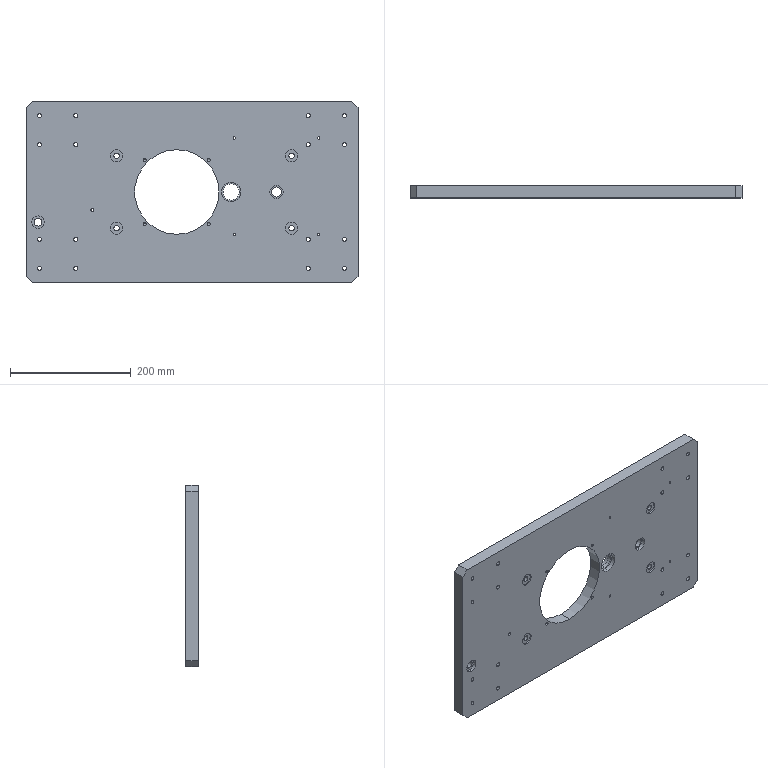Part | NX | features BREP 1 | 1 solid | 178 faces | box 550 x 20 x 300 mm | volume 2934740 mm3 | cylinder 120 | cone 34 | plane 24 | commonest cylinder face diameters 6.8 x32 2.5 x20 5 x16 4 x8 9 x8 15 x8